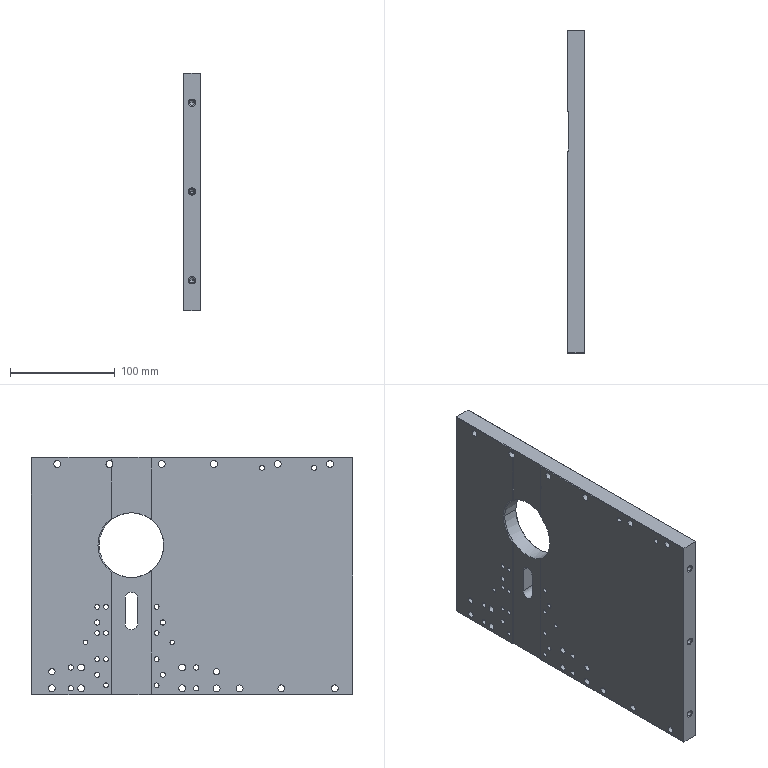Part | NX | 1 solid | 322 faces | box 17 x 308 x 227 mm | volume 1096361 mm3 | cylinder 179 | cone 92 | plane 51 | commonest cylinder face diameters 6.6 x30 11 x30 5 x26 3.3 x24 4.5 x22 8 x22